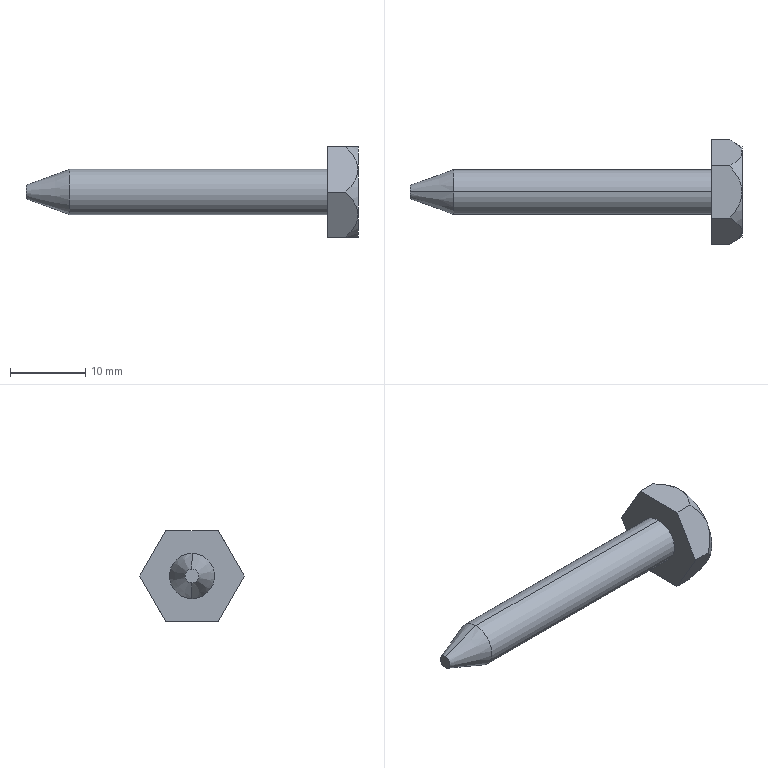Part | SolidWorks | features Extrusion 1, ICE 1, Revolution 1 | 1 solid | 19 faces | box 44 x 13.856 x 12 mm | volume 1537 mm3 | plane 9 | cone 8 | cylinder 2 | commonest cylinder face diameters 6 x2
STEP:
#1=CARTESIAN_POINT('',(-40.,0.,0.9));
#2=VERTEX_POINT('',#1);
#3=CARTESIAN_POINT('',(-40.,0.,-0.9));
#4=VERTEX_POINT('',#3);
#5=CARTESIAN_POINT('',(-40.,0.,0.));
#6=DIRECTION('',(-1.,0.,0.));
#7=DIRECTION('',(0.,0.,1.));
#8=AXIS2_PLACEMENT_3D('',#5,#6,#7);
#9=CIRCLE('',#8,0.9);
#10=EDGE_CURVE('',#2,#4,#9,.T.);
#11=ORIENTED_EDGE('',*,*,#10,.F.);
#12=CARTESIAN_POINT('',(-34.23,0.,3.));
#13=VERTEX_POINT('',#12);
#14=CARTESIAN_POINT('',(-34.23,0.,3.));
#15=DIRECTION('',(0.9397,0.,0.342));
#16=VECTOR('',#15,1000.);
#17=LINE('',#14,#16);
#18=EDGE_CURVE('',#2,#13,#17,.T.);
#19=ORIENTED_EDGE('',*,*,#18,.T.);
#20=CARTESIAN_POINT('',(-34.23,0.,-3.));
#21=VERTEX_POINT('',#20);
#22=CARTESIAN_POINT('',(-34.23,0.,0.));
#23=DIRECTION('',(-1.,0.,0.));
#24=DIRECTION('',(0.,0.,1.));
#25=AXIS2_PLACEMENT_3D('',#22,#23,#24);
#26=CIRCLE('',#25,3.);
#27=EDGE_CURVE('',#13,#21,#26,.T.);
#28=ORIENTED_EDGE('',*,*,#27,.T.);
#29=CARTESIAN_POINT('',(-34.23,0.,-3.));
#30=DIRECTION('',(0.9397,0.,-0.342));
#31=VECTOR('',#30,1000.);
#32=LINE('',#29,#31);
#33=EDGE_CURVE('',#4,#21,#32,.T.);
#34=ORIENTED_EDGE('',*,*,#33,.F.);
#35=EDGE_LOOP('',(#11,#19,#28,#34));
#36=FACE_OUTER_BOUND('',#35,.T.);
#37=CARTESIAN_POINT('',(-34.23,0.,0.));
#38=DIRECTION('',(1.,0.,0.));
#39=DIRECTION('',(0.,0.,-1.));
#40=AXIS2_PLACEMENT_3D('',#37,#38,#39);
#41=CONICAL_SURFACE('',#40,3.,0.3491);
#42=ADVANCED_FACE('',(#36),#41,.T.);
#43=CARTESIAN_POINT('',(0.,0.,3.));
#44=VERTEX_POINT('',#43);
#45=CARTESIAN_POINT('',(0.,0.,-3.));
#46=VERTEX_POINT('',#45);
#47=CARTESIAN_POINT('',(0.,0.,0.));
#48=DIRECTION('',(-1.,0.,0.));
#49=DIRECTION('',(0.,0.,1.));
#50=AXIS2_PLACEMENT_3D('',#47,#48,#49);
#51=CIRCLE('',#50,3.);
#52=EDGE_CURVE('',#44,#46,#51,.T.);
#53=ORIENTED_EDGE('',*,*,#52,.T.);
#54=CARTESIAN_POINT('',(-29.866,0.,-3.));
#55=DIRECTION('',(-1.,0.,0.));
#56=VECTOR('',#55,1000.);
#57=LINE('',#54,#56);
#58=EDGE_CURVE('',#46,#21,#57,.T.);
#59=ORIENTED_EDGE('',*,*,#58,.T.);
#60=ORIENTED_EDGE('',*,*,#27,.F.);
#61=CARTESIAN_POINT('',(-29.866,0.,3.));
#62=DIRECTION('',(-1.,0.,0.));
#63=VECTOR('',#62,1000.);
#64=LINE('',#61,#63);
#65=EDGE_CURVE('',#44,#13,#64,.T.);
#66=ORIENTED_EDGE('',*,*,#65,.F.);
#67=EDGE_LOOP('',(#53,#59,#60,#66));
#68=FACE_OUTER_BOUND('',#67,.T.);
#69=CARTESIAN_POINT('',(-29.866,0.,0.));
#70=DIRECTION('',(-1.,0.,0.));
#71=DIRECTION('',(0.,0.,1.));
#72=AXIS2_PLACEMENT_3D('',#69,#70,#71);
#73=CYLINDRICAL_SURFACE('',#72,3.);
#74=ADVANCED_FACE('',(#68),#73,.T.);
#75=CARTESIAN_POINT('',(2.392,-3.464,6.));
#76=VERTEX_POINT('',#75);
#77=CARTESIAN_POINT('',(4.,-5.196,3.));
#78=VERTEX_POINT('',#77);
#79=CARTESIAN_POINT('',(2.392,-3.464,6.));
#80=CARTESIAN_POINT('',(2.819,-3.711,5.573));
#81=CARTESIAN_POINT('',(3.206,-3.97,5.124));
#82=CARTESIAN_POINT('',(3.654,-4.403,4.374));
#83=CARTESIAN_POINT('',(3.78,-4.556,4.109));
#84=CARTESIAN_POINT('',(3.909,-4.791,3.702));
#85=CARTESIAN_POINT('',(3.943,-4.87,3.564));
#86=CARTESIAN_POINT('',(3.988,-5.032,3.284));
#87=CARTESIAN_POINT('',(4.,-5.115,3.141));
#88=CARTESIAN_POINT('',(4.,-5.196,3.));
#89=B_SPLINE_CURVE_WITH_KNOTS('',3,(#79,#80,#81,#82,#83,#84,#85,#86,#87,#88),.UNSPECIFIED.,.F.,.F.,(4,2,2,2,4),(0.000000303,0.001939,0.002909,0.003393,0.003878),.UNSPECIFIED.);
#90=EDGE_CURVE('',#76,#78,#89,.T.);
#91=ORIENTED_EDGE('',*,*,#90,.F.);
#92=CARTESIAN_POINT('',(0.,-3.464,6.));
#93=VERTEX_POINT('',#92);
#94=CARTESIAN_POINT('',(4.,-3.464,6.));
#95=DIRECTION('',(-1.,0.,0.));
#96=VECTOR('',#95,1000.);
#97=LINE('',#94,#96);
#98=EDGE_CURVE('',#76,#93,#97,.T.);
#99=ORIENTED_EDGE('',*,*,#98,.T.);
#100=CARTESIAN_POINT('',(0.,-6.928,0.));
#101=VERTEX_POINT('',#100);
#102=CARTESIAN_POINT('',(0.,-3.464,6.));
#103=DIRECTION('',(0.,-0.5,-0.866));
#104=VECTOR('',#103,1000.);
#105=LINE('',#102,#104);
#106=EDGE_CURVE('',#93,#101,#105,.T.);
#107=ORIENTED_EDGE('',*,*,#106,.T.);
#108=CARTESIAN_POINT('',(2.392,-6.928,0.));
#109=VERTEX_POINT('',#108);
#110=CARTESIAN_POINT('',(4.,-6.928,0.));
#111=DIRECTION('',(-1.,0.,0.));
#112=VECTOR('',#111,1000.);
#113=LINE('',#110,#112);
#114=EDGE_CURVE('',#109,#101,#113,.T.);
#115=ORIENTED_EDGE('',*,*,#114,.F.);
#116=CARTESIAN_POINT('',(4.,-5.196,3.));
#117=CARTESIAN_POINT('',(4.,-5.359,2.718));
#118=CARTESIAN_POINT('',(3.954,-5.519,2.441));
#119=CARTESIAN_POINT('',(3.781,-5.835,1.893));
#120=CARTESIAN_POINT('',(3.657,-5.985,1.633));
#121=CARTESIAN_POINT('',(3.361,-6.273,1.135));
#122=CARTESIAN_POINT('',(3.187,-6.412,0.8948));
#123=CARTESIAN_POINT('',(2.81,-6.678,0.4342));
#124=CARTESIAN_POINT('',(2.606,-6.805,0.2137));
#125=CARTESIAN_POINT('',(2.392,-6.928,0.));
#126=B_SPLINE_CURVE_WITH_KNOTS('',3,(#116,#117,#118,#119,#120,#121,#122,#123,#124,#125),.UNSPECIFIED.,.F.,.F.,(4,2,2,2,4),(0.003878,0.004846,0.005814,0.006782,0.00775),.UNSPECIFIED.);
#127=EDGE_CURVE('',#78,#109,#126,.T.);
#128=ORIENTED_EDGE('',*,*,#127,.F.);
#129=EDGE_LOOP('',(#91,#99,#107,#115,#128));
#130=FACE_OUTER_BOUND('',#129,.T.);
#131=CARTESIAN_POINT('',(4.,-3.464,6.));
#132=DIRECTION('',(0.,0.866,-0.5));
#133=DIRECTION('',(0.,0.5,0.866));
#134=AXIS2_PLACEMENT_3D('',#131,#132,#133);
#135=PLANE('',#134);
#136=ADVANCED_FACE('',(#130),#135,.F.);
#137=CARTESIAN_POINT('',(4.,-5.196,-3.));
#138=VERTEX_POINT('',#137);
#139=CARTESIAN_POINT('',(2.392,-6.928,0.));
#140=CARTESIAN_POINT('',(2.819,-6.682,-0.4268));
#141=CARTESIAN_POINT('',(3.206,-6.422,-0.8763));
#142=CARTESIAN_POINT('',(3.654,-5.989,-1.626));
#143=CARTESIAN_POINT('',(3.78,-5.836,-1.891));
#144=CARTESIAN_POINT('',(3.909,-5.601,-2.298));
#145=CARTESIAN_POINT('',(3.943,-5.522,-2.436));
#146=CARTESIAN_POINT('',(3.988,-5.36,-2.716));
#147=CARTESIAN_POINT('',(4.,-5.278,-2.859));
#148=CARTESIAN_POINT('',(4.,-5.196,-3.));
#149=B_SPLINE_CURVE_WITH_KNOTS('',3,(#139,#140,#141,#142,#143,#144,#145,#146,#147,#148),.UNSPECIFIED.,.F.,.F.,(4,2,2,2,4),(0.000000303,0.001939,0.002909,0.003393,0.003878),.UNSPECIFIED.);
#150=EDGE_CURVE('',#109,#138,#149,.T.);
#151=ORIENTED_EDGE('',*,*,#150,.F.);
#152=ORIENTED_EDGE('',*,*,#114,.T.);
#153=CARTESIAN_POINT('',(0.,-3.464,-6.));
#154=VERTEX_POINT('',#153);
#155=CARTESIAN_POINT('',(0.,-6.928,0.));
#156=DIRECTION('',(0.,0.5,-0.866));
#157=VECTOR('',#156,1000.);
#158=LINE('',#155,#157);
#159=EDGE_CURVE('',#101,#154,#158,.T.);
#160=ORIENTED_EDGE('',*,*,#159,.T.);
#161=CARTESIAN_POINT('',(2.392,-3.464,-6.));
#162=VERTEX_POINT('',#161);
#163=CARTESIAN_POINT('',(4.,-3.464,-6.));
#164=DIRECTION('',(-1.,0.,0.));
#165=VECTOR('',#164,1000.);
#166=LINE('',#163,#165);
#167=EDGE_CURVE('',#162,#154,#166,.T.);
#168=ORIENTED_EDGE('',*,*,#167,.F.);
#169=CARTESIAN_POINT('',(4.,-5.196,-3.));
#170=CARTESIAN_POINT('',(4.,-5.034,-3.282));
#171=CARTESIAN_POINT('',(3.954,-4.873,-3.559));
#172=CARTESIAN_POINT('',(3.781,-4.557,-4.107));
#173=CARTESIAN_POINT('',(3.657,-4.407,-4.367));
#174=CARTESIAN_POINT('',(3.361,-4.119,-4.865));
#175=CARTESIAN_POINT('',(3.187,-3.981,-5.105));
#176=CARTESIAN_POINT('',(2.81,-3.715,-5.566));
#177=CARTESIAN_POINT('',(2.606,-3.587,-5.786));
#178=CARTESIAN_POINT('',(2.392,-3.464,-6.));
#179=B_SPLINE_CURVE_WITH_KNOTS('',3,(#169,#170,#171,#172,#173,#174,#175,#176,#177,#178),.UNSPECIFIED.,.F.,.F.,(4,2,2,2,4),(0.003878,0.004846,0.005814,0.006782,0.00775),.UNSPECIFIED.);
#180=EDGE_CURVE('',#138,#162,#179,.T.);
#181=ORIENTED_EDGE('',*,*,#180,.F.);
#182=EDGE_LOOP('',(#151,#152,#160,#168,#181));
#183=FACE_OUTER_BOUND('',#182,.T.);
#184=CARTESIAN_POINT('',(4.,-6.928,0.));
#185=DIRECTION('',(0.,0.866,0.5));
#186=DIRECTION('',(0.,-0.5,0.866));
#187=AXIS2_PLACEMENT_3D('',#184,#185,#186);
#188=PLANE('',#187);
#189=ADVANCED_FACE('',(#183),#188,.F.);
#190=CARTESIAN_POINT('',(4.,0.,-6.));
#191=VERTEX_POINT('',#190);
#192=CARTESIAN_POINT('',(2.392,-3.464,-6.));
#193=CARTESIAN_POINT('',(2.604,-3.219,-6.));
#194=CARTESIAN_POINT('',(2.807,-2.967,-6.));
#195=CARTESIAN_POINT('',(3.183,-2.437,-6.));
#196=CARTESIAN_POINT('',(3.358,-2.158,-6.));
#197=CARTESIAN_POINT('',(3.657,-1.579,-6.));
#198=CARTESIAN_POINT('',(3.781,-1.278,-6.));
#199=CARTESIAN_POINT('',(3.954,-0.6439,-6.));
#200=CARTESIAN_POINT('',(4.,-0.3237,-6.));
#201=CARTESIAN_POINT('',(4.,0.,-6.));
#202=B_SPLINE_CURVE_WITH_KNOTS('',3,(#192,#193,#194,#195,#196,#197,#198,#199,#200,#201),.UNSPECIFIED.,.F.,.F.,(4,2,2,2,4),(0.01314,0.01411,0.01509,0.01606,0.01704),.UNSPECIFIED.);
#203=EDGE_CURVE('',#162,#191,#202,.T.);
#204=ORIENTED_EDGE('',*,*,#203,.F.);
#205=ORIENTED_EDGE('',*,*,#167,.T.);
#206=CARTESIAN_POINT('',(0.,3.464,-6.));
#207=VERTEX_POINT('',#206);
#208=CARTESIAN_POINT('',(0.,-3.464,-6.));
#209=DIRECTION('',(0.,1.,0.));
#210=VECTOR('',#209,1000.);
#211=LINE('',#208,#210);
#212=EDGE_CURVE('',#154,#207,#211,.T.);
#213=ORIENTED_EDGE('',*,*,#212,.T.);
#214=CARTESIAN_POINT('',(2.392,3.464,-6.));
#215=VERTEX_POINT('',#214);
#216=CARTESIAN_POINT('',(4.,3.464,-6.));
#217=DIRECTION('',(-1.,0.,0.));
#218=VECTOR('',#217,1000.);
#219=LINE('',#216,#218);
#220=EDGE_CURVE('',#215,#207,#219,.T.);
#221=ORIENTED_EDGE('',*,*,#220,.F.);
#222=CARTESIAN_POINT('',(4.,0.,-6.));
#223=CARTESIAN_POINT('',(4.,0.3232,-6.));
#224=CARTESIAN_POINT('',(3.952,0.6524,-6.));
#225=CARTESIAN_POINT('',(3.78,1.279,-6.));
#226=CARTESIAN_POINT('',(3.655,1.584,-6.));
#227=CARTESIAN_POINT('',(3.207,2.452,-6.));
#228=CARTESIAN_POINT('',(2.819,2.972,-6.));
#229=CARTESIAN_POINT('',(2.392,3.464,-6.));
#230=B_SPLINE_CURVE_WITH_KNOTS('',3,(#222,#223,#224,#225,#226,#227,#228,#229),.UNSPECIFIED.,.F.,.F.,(4,2,2,4),(0.01704,0.01801,0.01898,0.02093),.UNSPECIFIED.);
#231=EDGE_CURVE('',#191,#215,#230,.T.);
#232=ORIENTED_EDGE('',*,*,#231,.F.);
#233=EDGE_LOOP('',(#204,#205,#213,#221,#232));
#234=FACE_OUTER_BOUND('',#233,.T.);
#235=CARTESIAN_POINT('',(4.,-3.464,-6.));
#236=DIRECTION('',(0.,0.,1.));
#237=DIRECTION('',(0.,-1.,0.));
#238=AXIS2_PLACEMENT_3D('',#235,#236,#237);
#239=PLANE('',#238);
#240=ADVANCED_FACE('',(#234),#239,.F.);
#241=CARTESIAN_POINT('',(4.,5.196,-3.));
#242=VERTEX_POINT('',#241);
#243=CARTESIAN_POINT('',(2.392,3.464,-6.));
#244=CARTESIAN_POINT('',(2.819,3.711,-5.573));
#245=CARTESIAN_POINT('',(3.206,3.97,-5.124));
#246=CARTESIAN_POINT('',(3.654,4.403,-4.374));
#247=CARTESIAN_POINT('',(3.78,4.556,-4.109));
#248=CARTESIAN_POINT('',(3.909,4.791,-3.702));
#249=CARTESIAN_POINT('',(3.943,4.87,-3.564));
#250=CARTESIAN_POINT('',(3.988,5.032,-3.284));
#251=CARTESIAN_POINT('',(4.,5.115,-3.141));
#252=CARTESIAN_POINT('',(4.,5.196,-3.));
#253=B_SPLINE_CURVE_WITH_KNOTS('',3,(#243,#244,#245,#246,#247,#248,#249,#250,#251,#252),.UNSPECIFIED.,.F.,.F.,(4,2,2,2,4),(0.000000303,0.001939,0.002909,0.003393,0.003878),.UNSPECIFIED.);
#254=EDGE_CURVE('',#215,#242,#253,.T.);
#255=ORIENTED_EDGE('',*,*,#254,.F.);
#256=ORIENTED_EDGE('',*,*,#220,.T.);
#257=CARTESIAN_POINT('',(0.,6.928,0.));
#258=VERTEX_POINT('',#257);
#259=CARTESIAN_POINT('',(0.,3.464,-6.));
#260=DIRECTION('',(0.,0.5,0.866));
#261=VECTOR('',#260,1000.);
#262=LINE('',#259,#261);
#263=EDGE_CURVE('',#207,#258,#262,.T.);
#264=ORIENTED_EDGE('',*,*,#263,.T.);
#265=CARTESIAN_POINT('',(2.392,6.928,0.));
#266=VERTEX_POINT('',#265);
#267=CARTESIAN_POINT('',(4.,6.928,0.));
#268=DIRECTION('',(-1.,0.,0.));
#269=VECTOR('',#268,1000.);
#270=LINE('',#267,#269);
#271=EDGE_CURVE('',#266,#258,#270,.T.);
#272=ORIENTED_EDGE('',*,*,#271,.F.);
#273=CARTESIAN_POINT('',(4.,5.196,-3.));
#274=CARTESIAN_POINT('',(4.,5.359,-2.718));
#275=CARTESIAN_POINT('',(3.954,5.519,-2.441));
#276=CARTESIAN_POINT('',(3.781,5.835,-1.893));
#277=CARTESIAN_POINT('',(3.657,5.985,-1.633));
#278=CARTESIAN_POINT('',(3.361,6.273,-1.135));
#279=CARTESIAN_POINT('',(3.187,6.412,-0.8948));
#280=CARTESIAN_POINT('',(2.81,6.678,-0.4342));
#281=CARTESIAN_POINT('',(2.606,6.805,-0.2137));
#282=CARTESIAN_POINT('',(2.392,6.928,0.));
#283=B_SPLINE_CURVE_WITH_KNOTS('',3,(#273,#274,#275,#276,#277,#278,#279,#280,#281,#282),.UNSPECIFIED.,.F.,.F.,(4,2,2,2,4),(0.003878,0.004846,0.005814,0.006782,0.00775),.UNSPECIFIED.);
#284=EDGE_CURVE('',#242,#266,#283,.T.);
#285=ORIENTED_EDGE('',*,*,#284,.F.);
#286=EDGE_LOOP('',(#255,#256,#264,#272,#285));
#287=FACE_OUTER_BOUND('',#286,.T.);
#288=CARTESIAN_POINT('',(4.,3.464,-6.));
#289=DIRECTION('',(0.,-0.866,0.5));
#290=DIRECTION('',(0.,-0.5,-0.866));
#291=AXIS2_PLACEMENT_3D('',#288,#289,#290);
#292=PLANE('',#291);
#293=ADVANCED_FACE('',(#287),#292,.F.);
#294=CARTESIAN_POINT('',(4.,5.196,3.));
#295=VERTEX_POINT('',#294);
#296=CARTESIAN_POINT('',(2.392,6.928,0.));
#297=CARTESIAN_POINT('',(2.819,6.682,0.4268));
#298=CARTESIAN_POINT('',(3.206,6.422,0.8763));
#299=CARTESIAN_POINT('',(3.654,5.989,1.626));
#300=CARTESIAN_POINT('',(3.78,5.836,1.891));
#301=CARTESIAN_POINT('',(3.909,5.601,2.298));
#302=CARTESIAN_POINT('',(3.943,5.522,2.436));
#303=CARTESIAN_POINT('',(3.988,5.36,2.716));
#304=CARTESIAN_POINT('',(4.,5.278,2.859));
#305=CARTESIAN_POINT('',(4.,5.196,3.));
#306=B_SPLINE_CURVE_WITH_KNOTS('',3,(#296,#297,#298,#299,#300,#301,#302,#303,#304,#305),.UNSPECIFIED.,.F.,.F.,(4,2,2,2,4),(0.000000303,0.001939,0.002909,0.003393,0.003878),.UNSPECIFIED.);
#307=EDGE_CURVE('',#266,#295,#306,.T.);
#308=ORIENTED_EDGE('',*,*,#307,.F.);
#309=ORIENTED_EDGE('',*,*,#271,.T.);
#310=CARTESIAN_POINT('',(0.,3.464,6.));
#311=VERTEX_POINT('',#310);
#312=CARTESIAN_POINT('',(0.,6.928,0.));
#313=DIRECTION('',(0.,-0.5,0.866));
#314=VECTOR('',#313,1000.);
#315=LINE('',#312,#314);
#316=EDGE_CURVE('',#258,#311,#315,.T.);
#317=ORIENTED_EDGE('',*,*,#316,.T.);
#318=CARTESIAN_POINT('',(2.392,3.464,6.));
#319=VERTEX_POINT('',#318);
#320=CARTESIAN_POINT('',(4.,3.464,6.));
#321=DIRECTION('',(-1.,0.,0.));
#322=VECTOR('',#321,1000.);
#323=LINE('',#320,#322);
#324=EDGE_CURVE('',#319,#311,#323,.T.);
#325=ORIENTED_EDGE('',*,*,#324,.F.);
#326=CARTESIAN_POINT('',(4.,5.196,3.));
#327=CARTESIAN_POINT('',(4.,5.034,3.282));
#328=CARTESIAN_POINT('',(3.954,4.873,3.559));
#329=CARTESIAN_POINT('',(3.781,4.557,4.107));
#330=CARTESIAN_POINT('',(3.657,4.407,4.367));
#331=CARTESIAN_POINT('',(3.361,4.119,4.865));
#332=CARTESIAN_POINT('',(3.187,3.981,5.105));
#333=CARTESIAN_POINT('',(2.81,3.715,5.566));
#334=CARTESIAN_POINT('',(2.606,3.587,5.786));
#335=CARTESIAN_POINT('',(2.392,3.464,6.));
#336=B_SPLINE_CURVE_WITH_KNOTS('',3,(#326,#327,#328,#329,#330,#331,#332,#333,#334,#335),.UNSPECIFIED.,.F.,.F.,(4,2,2,2,4),(0.003878,0.004846,0.005814,0.006782,0.00775),.UNSPECIFIED.);
#337=EDGE_CURVE('',#295,#319,#336,.T.);
#338=ORIENTED_EDGE('',*,*,#337,.F.);
#339=EDGE_LOOP('',(#308,#309,#317,#325,#338));
#340=FACE_OUTER_BOUND('',#339,.T.);
#341=CARTESIAN_POINT('',(4.,6.928,0.));
#342=DIRECTION('',(0.,-0.866,-0.5));
#343=DIRECTION('',(0.,0.5,-0.866));
#344=AXIS2_PLACEMENT_3D('',#341,#342,#343);
#345=PLANE('',#344);
#346=ADVANCED_FACE('',(#340),#345,.F.);
#347=CARTESIAN_POINT('',(4.,0.,6.));
#348=VERTEX_POINT('',#347);
#349=CARTESIAN_POINT('',(2.392,3.464,6.));
#350=CARTESIAN_POINT('',(2.604,3.219,6.));
#351=CARTESIAN_POINT('',(2.807,2.967,6.));
#352=CARTESIAN_POINT('',(3.183,2.437,6.));
#353=CARTESIAN_POINT('',(3.358,2.158,6.));
#354=CARTESIAN_POINT('',(3.657,1.579,6.));
#355=CARTESIAN_POINT('',(3.781,1.278,6.));
#356=CARTESIAN_POINT('',(3.954,0.6439,6.));
#357=CARTESIAN_POINT('',(4.,0.3237,6.));
#358=CARTESIAN_POINT('',(4.,0.,6.));
#359=B_SPLINE_CURVE_WITH_KNOTS('',3,(#349,#350,#351,#352,#353,#354,#355,#356,#357,#358),.UNSPECIFIED.,.F.,.F.,(4,2,2,2,4),(0.01314,0.01411,0.01509,0.01606,0.01704),.UNSPECIFIED.);
#360=EDGE_CURVE('',#319,#348,#359,.T.);
#361=ORIENTED_EDGE('',*,*,#360,.F.);
#362=ORIENTED_EDGE('',*,*,#324,.T.);
#363=CARTESIAN_POINT('',(0.,3.464,6.));
#364=DIRECTION('',(0.,-1.,0.));
#365=VECTOR('',#364,1000.);
#366=LINE('',#363,#365);
#367=EDGE_CURVE('',#311,#93,#366,.T.);
#368=ORIENTED_EDGE('',*,*,#367,.T.);
#369=ORIENTED_EDGE('',*,*,#98,.F.);
#370=CARTESIAN_POINT('',(4.,0.,6.));
#371=CARTESIAN_POINT('',(4.,-0.3232,6.));
#372=CARTESIAN_POINT('',(3.952,-0.6524,6.));
#373=CARTESIAN_POINT('',(3.78,-1.279,6.));
#374=CARTESIAN_POINT('',(3.655,-1.584,6.));
#375=CARTESIAN_POINT('',(3.207,-2.452,6.));
#376=CARTESIAN_POINT('',(2.819,-2.972,6.));
#377=CARTESIAN_POINT('',(2.392,-3.464,6.));
#378=B_SPLINE_CURVE_WITH_KNOTS('',3,(#370,#371,#372,#373,#374,#375,#376,#377),.UNSPECIFIED.,.F.,.F.,(4,2,2,4),(0.01704,0.01801,0.01898,0.02093),.UNSPECIFIED.);
#379=EDGE_CURVE('',#348,#76,#378,.T.);
#380=ORIENTED_EDGE('',*,*,#379,.F.);
#381=EDGE_LOOP('',(#361,#362,#368,#369,#380));
#382=FACE_OUTER_BOUND('',#381,.T.);
#383=CARTESIAN_POINT('',(4.,3.464,6.));
#384=DIRECTION('',(0.,0.,-1.));
#385=DIRECTION('',(0.,1.,0.));
#386=AXIS2_PLACEMENT_3D('',#383,#384,#385);
#387=PLANE('',#386);
#388=ADVANCED_FACE('',(#382),#387,.F.);
#389=ORIENTED_EDGE('',*,*,#52,.F.);
#390=CARTESIAN_POINT('',(0.,0.,0.));
#391=DIRECTION('',(-1.,0.,0.));
#392=DIRECTION('',(0.,0.,1.));
#393=AXIS2_PLACEMENT_3D('',#390,#391,#392);
#394=CIRCLE('',#393,3.);
#395=EDGE_CURVE('',#46,#44,#394,.T.);
#396=ORIENTED_EDGE('',*,*,#395,.F.);
#397=EDGE_LOOP('',(#389,#396));
#398=FACE_BOUND('',#397,.T.);
#399=ORIENTED_EDGE('',*,*,#106,.F.);
#400=ORIENTED_EDGE('',*,*,#367,.F.);
#401=ORIENTED_EDGE('',*,*,#316,.F.);
#402=ORIENTED_EDGE('',*,*,#263,.F.);
#403=ORIENTED_EDGE('',*,*,#212,.F.);
#404=ORIENTED_EDGE('',*,*,#159,.F.);
#405=EDGE_LOOP('',(#399,#400,#401,#402,#403,#404));
#406=FACE_OUTER_BOUND('',#405,.T.);
#407=CARTESIAN_POINT('',(0.,0.,0.));
#408=DIRECTION('',(1.,0.,0.));
#409=DIRECTION('',(0.,0.,-1.));
#410=AXIS2_PLACEMENT_3D('',#407,#408,#409);
#411=PLANE('',#410);
#412=ADVANCED_FACE('',(#398,#406),#411,.F.);
#413=ORIENTED_EDGE('',*,*,#180,.T.);
#414=ORIENTED_EDGE('',*,*,#203,.T.);
#415=CARTESIAN_POINT('',(4.,0.,0.));
#416=DIRECTION('',(1.,0.,0.));
#417=DIRECTION('',(0.,0.,-1.));
#418=AXIS2_PLACEMENT_3D('',#415,#416,#417);
#419=CIRCLE('',#418,6.);
#420=EDGE_CURVE('',#138,#191,#419,.T.);
#421=ORIENTED_EDGE('',*,*,#420,.F.);
#422=EDGE_LOOP('',(#413,#414,#421));
#423=FACE_OUTER_BOUND('',#422,.T.);
#424=CARTESIAN_POINT('',(4.,0.,0.));
#425=DIRECTION('',(-1.,0.,0.));
#426=DIRECTION('',(0.,0.,-1.));
#427=AXIS2_PLACEMENT_3D('',#424,#425,#426);
#428=CONICAL_SURFACE('',#427,6.,0.5236);
#429=ADVANCED_FACE('',(#423),#428,.T.);
#430=ORIENTED_EDGE('',*,*,#127,.T.);
#431=ORIENTED_EDGE('',*,*,#150,.T.);
#432=CARTESIAN_POINT('',(4.,0.,0.));
#433=DIRECTION('',(1.,0.,0.));
#434=DIRECTION('',(0.,0.,-1.));
#435=AXIS2_PLACEMENT_3D('',#432,#433,#434);
#436=CIRCLE('',#435,6.);
#437=EDGE_CURVE('',#78,#138,#436,.T.);
#438=ORIENTED_EDGE('',*,*,#437,.F.);
#439=EDGE_LOOP('',(#430,#431,#438));
#440=FACE_OUTER_BOUND('',#439,.T.);
#441=CARTESIAN_POINT('',(4.,0.,0.));
#442=DIRECTION('',(-1.,0.,0.));
#443=DIRECTION('',(0.,0.,-1.));
#444=AXIS2_PLACEMENT_3D('',#441,#442,#443);
#445=CONICAL_SURFACE('',#444,6.,0.5236);
#446=ADVANCED_FACE('',(#440),#445,.T.);
#447=ORIENTED_EDGE('',*,*,#90,.T.);
#448=CARTESIAN_POINT('',(4.,0.,0.));
#449=DIRECTION('',(1.,0.,0.));
#450=DIRECTION('',(0.,0.,-1.));
#451=AXIS2_PLACEMENT_3D('',#448,#449,#450);
#452=CIRCLE('',#451,6.);
#453=EDGE_CURVE('',#348,#78,#452,.T.);
#454=ORIENTED_EDGE('',*,*,#453,.F.);
#455=ORIENTED_EDGE('',*,*,#379,.T.);
#456=EDGE_LOOP('',(#447,#454,#455));
#457=FACE_OUTER_BOUND('',#456,.T.);
#458=CARTESIAN_POINT('',(4.,0.,0.));
#459=DIRECTION('',(-1.,0.,0.));
#460=DIRECTION('',(0.,0.,-1.));
#461=AXIS2_PLACEMENT_3D('',#458,#459,#460);
#462=CONICAL_SURFACE('',#461,6.,0.5236);
#463=ADVANCED_FACE('',(#457),#462,.T.);
#464=ORIENTED_EDGE('',*,*,#337,.T.);
#465=ORIENTED_EDGE('',*,*,#360,.T.);
#466=CARTESIAN_POINT('',(4.,0.,0.));
#467=DIRECTION('',(1.,0.,0.));
#468=DIRECTION('',(0.,0.,-1.));
#469=AXIS2_PLACEMENT_3D('',#466,#467,#468);
#470=CIRCLE('',#469,6.);
#471=EDGE_CURVE('',#295,#348,#470,.T.);
#472=ORIENTED_EDGE('',*,*,#471,.F.);
#473=EDGE_LOOP('',(#464,#465,#472));
#474=FACE_OUTER_BOUND('',#473,.T.);
#475=CARTESIAN_POINT('',(4.,0.,0.));
#476=DIRECTION('',(-1.,0.,0.));
#477=DIRECTION('',(0.,0.,-1.));
#478=AXIS2_PLACEMENT_3D('',#475,#476,#477);
#479=CONICAL_SURFACE('',#478,6.,0.5236);
#480=ADVANCED_FACE('',(#474),#479,.T.);
#481=ORIENTED_EDGE('',*,*,#284,.T.);
#482=ORIENTED_EDGE('',*,*,#307,.T.);
#483=CARTESIAN_POINT('',(4.,0.,0.));
#484=DIRECTION('',(1.,0.,0.));
#485=DIRECTION('',(0.,0.,-1.));
#486=AXIS2_PLACEMENT_3D('',#483,#484,#485);
#487=CIRCLE('',#486,6.);
#488=EDGE_CURVE('',#242,#295,#487,.T.);
#489=ORIENTED_EDGE('',*,*,#488,.F.);
#490=EDGE_LOOP('',(#481,#482,#489));
#491=FACE_OUTER_BOUND('',#490,.T.);
#492=CARTESIAN_POINT('',(4.,0.,0.));
#493=DIRECTION('',(-1.,0.,0.));
#494=DIRECTION('',(0.,0.,-1.));
#495=AXIS2_PLACEMENT_3D('',#492,#493,#494);
#496=CONICAL_SURFACE('',#495,6.,0.5236);
#497=ADVANCED_FACE('',(#491),#496,.T.);
#498=ORIENTED_EDGE('',*,*,#231,.T.);
#499=ORIENTED_EDGE('',*,*,#254,.T.);
#500=CARTESIAN_POINT('',(4.,0.,0.));
#501=DIRECTION('',(1.,0.,0.));
#502=DIRECTION('',(0.,0.,-1.));
#503=AXIS2_PLACEMENT_3D('',#500,#501,#502);
#504=CIRCLE('',#503,6.);
#505=EDGE_CURVE('',#191,#242,#504,.T.);
#506=ORIENTED_EDGE('',*,*,#505,.F.);
#507=EDGE_LOOP('',(#498,#499,#506));
#508=FACE_OUTER_BOUND('',#507,.T.);
#509=CARTESIAN_POINT('',(4.,0.,0.));
#510=DIRECTION('',(-1.,0.,0.));
#511=DIRECTION('',(0.,0.,-1.));
#512=AXIS2_PLACEMENT_3D('',#509,#510,#511);
#513=CONICAL_SURFACE('',#512,6.,0.5236);
#514=ADVANCED_FACE('',(#508),#513,.T.);
#515=ORIENTED_EDGE('',*,*,#420,.T.);
#516=ORIENTED_EDGE('',*,*,#505,.T.);
#517=ORIENTED_EDGE('',*,*,#488,.T.);
#518=ORIENTED_EDGE('',*,*,#471,.T.);
#519=ORIENTED_EDGE('',*,*,#453,.T.);
#520=ORIENTED_EDGE('',*,*,#437,.T.);
#521=EDGE_LOOP('',(#515,#516,#517,#518,#519,#520));
#522=FACE_OUTER_BOUND('',#521,.T.);
#523=CARTESIAN_POINT('',(4.,0.,0.));
#524=DIRECTION('',(1.,0.,0.));
#525=DIRECTION('',(0.,0.,-1.));
#526=AXIS2_PLACEMENT_3D('',#523,#524,#525);
#527=PLANE('',#526);
#528=ADVANCED_FACE('',(#522),#527,.T.);
#529=ORIENTED_EDGE('',*,*,#58,.F.);
#530=ORIENTED_EDGE('',*,*,#395,.T.);
#531=ORIENTED_EDGE('',*,*,#65,.T.);
#532=CARTESIAN_POINT('',(-34.23,0.,0.));
#533=DIRECTION('',(-1.,0.,0.));
#534=DIRECTION('',(0.,0.,1.));
#535=AXIS2_PLACEMENT_3D('',#532,#533,#534);
#536=CIRCLE('',#535,3.);
#537=EDGE_CURVE('',#21,#13,#536,.T.);
#538=ORIENTED_EDGE('',*,*,#537,.F.);
#539=EDGE_LOOP('',(#529,#530,#531,#538));
#540=FACE_OUTER_BOUND('',#539,.T.);
#541=CARTESIAN_POINT('',(-29.866,0.,0.));
#542=DIRECTION('',(-1.,0.,0.));
#543=DIRECTION('',(0.,0.,1.));
#544=AXIS2_PLACEMENT_3D('',#541,#542,#543);
#545=CYLINDRICAL_SURFACE('',#544,3.);
#546=ADVANCED_FACE('',(#540),#545,.T.);
#547=CARTESIAN_POINT('',(-40.,0.,0.));
#548=DIRECTION('',(-1.,0.,0.));
#549=DIRECTION('',(0.,0.,1.));
#550=AXIS2_PLACEMENT_3D('',#547,#548,#549);
#551=CIRCLE('',#550,0.9);
#552=EDGE_CURVE('',#4,#2,#551,.T.);
#553=ORIENTED_EDGE('',*,*,#552,.T.);
#554=ORIENTED_EDGE('',*,*,#10,.T.);
#555=EDGE_LOOP('',(#553,#554));
#556=FACE_OUTER_BOUND('',#555,.T.);
#557=CARTESIAN_POINT('',(-40.,0.,0.));
#558=DIRECTION('',(1.,0.,0.));
#559=DIRECTION('',(0.,0.,-1.));
#560=AXIS2_PLACEMENT_3D('',#557,#558,#559);
#561=PLANE('',#560);
#562=ADVANCED_FACE('',(#556),#561,.F.);
#563=ORIENTED_EDGE('',*,*,#18,.F.);
#564=ORIENTED_EDGE('',*,*,#552,.F.);
#565=ORIENTED_EDGE('',*,*,#33,.T.);
#566=ORIENTED_EDGE('',*,*,#537,.T.);
#567=EDGE_LOOP('',(#563,#564,#565,#566));
#568=FACE_OUTER_BOUND('',#567,.T.);
#569=CARTESIAN_POINT('',(-34.23,0.,0.));
#570=DIRECTION('',(1.,0.,0.));
#571=DIRECTION('',(0.,0.,-1.));
#572=AXIS2_PLACEMENT_3D('',#569,#570,#571);
#573=CONICAL_SURFACE('',#572,3.,0.3491);
#574=ADVANCED_FACE('',(#568),#573,.T.);
#575=CLOSED_SHELL('',(#42,#74,#136,#189,#240,#293,#346,#388,#412,#429,#446,#463,#480,#497,#514,#528,#546,#562,#574));
#576=MANIFOLD_SOLID_BREP('',#575);
#577=CARTESIAN_POINT('',(0.,0.,0.));
#578=DIRECTION('',(0.,0.,1.));
#579=DIRECTION('',(1.,0.,0.));
#580=AXIS2_PLACEMENT_3D('',#577,#578,#579);
#581=(LENGTH_UNIT()NAMED_UNIT(*)SI_UNIT(.MILLI.,.METRE.));
#582=UNCERTAINTY_MEASURE_WITH_UNIT(LENGTH_MEASURE(0.00001),#581,'','');
#583=(NAMED_UNIT(*)PLANE_ANGLE_UNIT()SI_UNIT($,.RADIAN.));
#584=(NAMED_UNIT(*)SI_UNIT($,.STERADIAN.)SOLID_ANGLE_UNIT());
#585=(GEOMETRIC_REPRESENTATION_CONTEXT(3)GLOBAL_UNCERTAINTY_ASSIGNED_CONTEXT((#582))GLOBAL_UNIT_ASSIGNED_CONTEXT((#581,#583,#584))REPRESENTATION_CONTEXT('',''));
#586=ADVANCED_BREP_SHAPE_REPRESENTATION('',(#576,#580),#585);